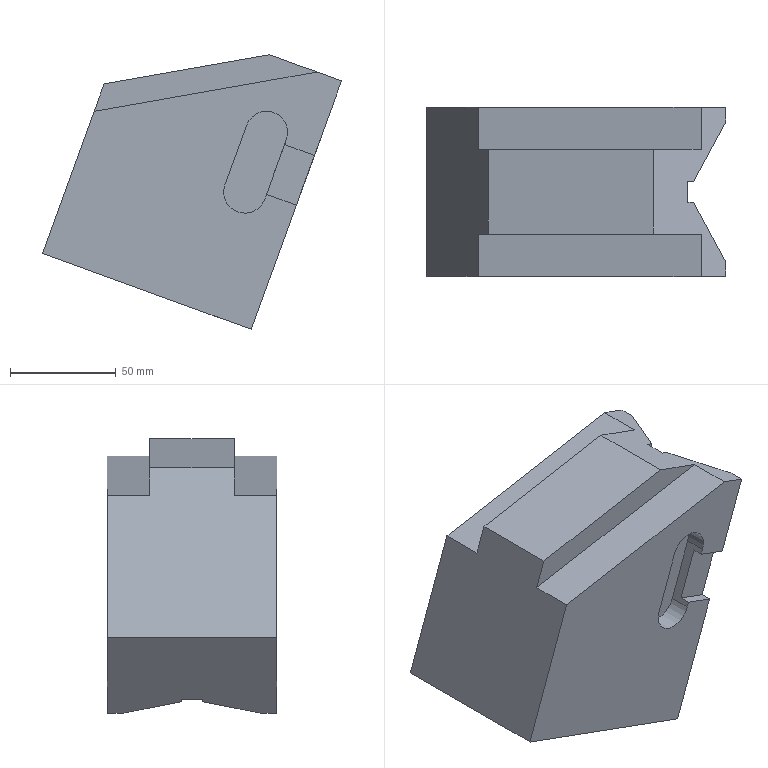Part | NX | features solid 2 | 1 solid | 33 faces | box 141.42 x 80 x 129.874 mm | volume 794242 mm3 | plane 29 | cylinder 4 | commonest cylinder face diameters 20 x4
STEP:
#1=CARTESIAN_POINT('',(813.449,-220.,121.531));
#2=VERTEX_POINT('',#1);
#3=CARTESIAN_POINT('',(828.59,-247.909,116.019));
#4=VERTEX_POINT('',#3);
#5=CARTESIAN_POINT('',(816.161,-225.,120.543));
#6=DIRECTION('',(0.4698,-0.866,-0.171));
#7=VECTOR('',#6,1000.);
#8=LINE('',#5,#7);
#9=EDGE_CURVE('',#2,#4,#8,.T.);
#10=ORIENTED_EDGE('',*,*,#9,.T.);
#11=CARTESIAN_POINT('',(785.838,-247.909,-1.442));
#12=VERTEX_POINT('',#11);
#13=CARTESIAN_POINT('',(837.141,-247.909,139.512));
#14=DIRECTION('',(-0.342,0.,-0.9397));
#15=VECTOR('',#14,1000.);
#16=LINE('',#13,#15);
#17=EDGE_CURVE('',#4,#12,#16,.T.);
#18=ORIENTED_EDGE('',*,*,#17,.T.);
#19=CARTESIAN_POINT('',(770.696,-220.,4.069));
#20=VERTEX_POINT('',#19);
#21=CARTESIAN_POINT('',(773.409,-225.,3.082));
#22=DIRECTION('',(0.4698,-0.866,-0.171));
#23=VECTOR('',#22,1000.);
#24=LINE('',#21,#23);
#25=EDGE_CURVE('',#20,#12,#24,.T.);
#26=ORIENTED_EDGE('',*,*,#25,.F.);
#27=CARTESIAN_POINT('',(821.999,-220.,145.023));
#28=DIRECTION('',(0.342,0.,0.9397));
#29=VECTOR('',#28,1000.);
#30=LINE('',#27,#29);
#31=EDGE_CURVE('',#20,#2,#30,.T.);
#32=ORIENTED_EDGE('',*,*,#31,.T.);
#33=EDGE_LOOP('',(#10,#18,#26,#32));
#34=FACE_BOUND('',#33,.T.);
#35=CARTESIAN_POINT('',(824.712,-225.,144.036));
#36=DIRECTION('',(0.8138,0.5,-0.2962));
#37=DIRECTION('',(0.342,0.,0.9397));
#38=AXIS2_PLACEMENT_3D('',#35,#36,#37);
#39=PLANE('',#38);
#40=ADVANCED_FACE('',(#34),#39,.T.);
#41=CARTESIAN_POINT('',(817.041,-175.,120.223));
#42=VERTEX_POINT('',#41);
#43=CARTESIAN_POINT('',(711.616,-175.,101.634));
#44=VERTEX_POINT('',#43);
#45=CARTESIAN_POINT('',(764.544,-175.,110.966));
#46=DIRECTION('',(-0.9848,0.,-0.1736));
#47=VECTOR('',#46,1000.);
#48=LINE('',#45,#47);
#49=EDGE_CURVE('',#42,#44,#48,.T.);
#50=ORIENTED_EDGE('',*,*,#49,.T.);
#51=CARTESIAN_POINT('',(711.616,-195.,101.634));
#52=VERTEX_POINT('',#51);
#53=CARTESIAN_POINT('',(711.616,-235.,101.634));
#54=DIRECTION('',(0.,1.,0.));
#55=VECTOR('',#54,1000.);
#56=LINE('',#53,#55);
#57=EDGE_CURVE('',#52,#44,#56,.T.);
#58=ORIENTED_EDGE('',*,*,#57,.F.);
#59=CARTESIAN_POINT('',(817.041,-195.,120.223));
#60=VERTEX_POINT('',#59);
#61=CARTESIAN_POINT('',(873.255,-195.,130.135));
#62=DIRECTION('',(0.9848,0.,0.1736));
#63=VECTOR('',#62,1000.);
#64=LINE('',#61,#63);
#65=EDGE_CURVE('',#60,#52,#64,.F.);
#66=ORIENTED_EDGE('',*,*,#65,.F.);
#67=CARTESIAN_POINT('',(817.041,-235.,120.223));
#68=DIRECTION('',(0.,-1.,0.));
#69=VECTOR('',#68,1000.);
#70=LINE('',#67,#69);
#71=EDGE_CURVE('',#42,#60,#70,.T.);
#72=ORIENTED_EDGE('',*,*,#71,.F.);
#73=EDGE_LOOP('',(#50,#58,#66,#72));
#74=FACE_BOUND('',#73,.T.);
#75=CARTESIAN_POINT('',(873.255,-235.,130.135));
#76=DIRECTION('',(0.1736,0.,-0.9848));
#77=DIRECTION('',(0.9848,0.,0.1736));
#78=AXIS2_PLACEMENT_3D('',#75,#76,#77);
#79=PLANE('',#78);
#80=ADVANCED_FACE('',(#74),#79,.F.);
#81=CARTESIAN_POINT('',(785.838,-175.,-1.442));
#82=VERTEX_POINT('',#81);
#83=CARTESIAN_POINT('',(687.17,-175.,34.47));
#84=VERTEX_POINT('',#83);
#85=CARTESIAN_POINT('',(781.139,-175.,0.268));
#86=DIRECTION('',(-0.9397,0.,0.342));
#87=VECTOR('',#86,1000.);
#88=LINE('',#85,#87);
#89=EDGE_CURVE('',#82,#84,#88,.T.);
#90=ORIENTED_EDGE('',*,*,#89,.F.);
#91=CARTESIAN_POINT('',(785.838,-182.091,-1.442));
#92=VERTEX_POINT('',#91);
#93=CARTESIAN_POINT('',(785.838,-175.,-1.442));
#94=DIRECTION('',(0.,1.,0.));
#95=VECTOR('',#94,1000.);
#96=LINE('',#93,#95);
#97=EDGE_CURVE('',#92,#82,#96,.T.);
#98=ORIENTED_EDGE('',*,*,#97,.F.);
#99=CARTESIAN_POINT('',(770.696,-210.,4.069));
#100=VERTEX_POINT('',#99);
#101=CARTESIAN_POINT('',(773.409,-205.,3.082));
#102=DIRECTION('',(0.4698,0.866,-0.171));
#103=VECTOR('',#102,1000.);
#104=LINE('',#101,#103);
#105=EDGE_CURVE('',#100,#92,#104,.T.);
#106=ORIENTED_EDGE('',*,*,#105,.F.);
#107=CARTESIAN_POINT('',(767.984,-210.,5.056));
#108=VERTEX_POINT('',#107);
#109=CARTESIAN_POINT('',(781.139,-210.,0.268));
#110=DIRECTION('',(0.9397,0.,-0.342));
#111=VECTOR('',#110,1000.);
#112=LINE('',#109,#111);
#113=EDGE_CURVE('',#108,#100,#112,.T.);
#114=ORIENTED_EDGE('',*,*,#113,.F.);
#115=CARTESIAN_POINT('',(767.984,-220.,5.056));
#116=VERTEX_POINT('',#115);
#117=CARTESIAN_POINT('',(767.984,-215.,5.056));
#118=DIRECTION('',(0.,1.,0.));
#119=VECTOR('',#118,1000.);
#120=LINE('',#117,#119);
#121=EDGE_CURVE('',#116,#108,#120,.T.);
#122=ORIENTED_EDGE('',*,*,#121,.F.);
#123=CARTESIAN_POINT('',(781.139,-220.,0.268));
#124=DIRECTION('',(0.9397,0.,-0.342));
#125=VECTOR('',#124,1000.);
#126=LINE('',#123,#125);
#127=EDGE_CURVE('',#116,#20,#126,.T.);
#128=ORIENTED_EDGE('',*,*,#127,.T.);
#129=ORIENTED_EDGE('',*,*,#25,.T.);
#130=CARTESIAN_POINT('',(785.838,-255.,-1.442));
#131=VERTEX_POINT('',#130);
#132=CARTESIAN_POINT('',(785.838,-255.,-1.442));
#133=DIRECTION('',(0.,-1.,0.));
#134=VECTOR('',#133,1000.);
#135=LINE('',#132,#134);
#136=EDGE_CURVE('',#12,#131,#135,.T.);
#137=ORIENTED_EDGE('',*,*,#136,.T.);
#138=CARTESIAN_POINT('',(687.17,-255.,34.47));
#139=VERTEX_POINT('',#138);
#140=CARTESIAN_POINT('',(781.139,-255.,0.268));
#141=DIRECTION('',(-0.9397,0.,0.342));
#142=VECTOR('',#141,1000.);
#143=LINE('',#140,#142);
#144=EDGE_CURVE('',#131,#139,#143,.T.);
#145=ORIENTED_EDGE('',*,*,#144,.T.);
#146=CARTESIAN_POINT('',(687.17,-215.,34.47));
#147=DIRECTION('',(0.,-1.,0.));
#148=VECTOR('',#147,1000.);
#149=LINE('',#146,#148);
#150=EDGE_CURVE('',#84,#139,#149,.T.);
#151=ORIENTED_EDGE('',*,*,#150,.F.);
#152=EDGE_LOOP('',(#90,#98,#106,#114,#122,#128,#129,#137,#145,#151));
#153=FACE_BOUND('',#152,.T.);
#154=CARTESIAN_POINT('',(781.139,-215.,0.268));
#155=DIRECTION('',(-0.342,0.,-0.9397));
#156=DIRECTION('',(0.9397,0.,-0.342));
#157=AXIS2_PLACEMENT_3D('',#154,#155,#156);
#158=PLANE('',#157);
#159=ADVANCED_FACE('',(#153),#158,.T.);
#160=CARTESIAN_POINT('',(817.041,-255.,120.223));
#161=VERTEX_POINT('',#160);
#162=CARTESIAN_POINT('',(711.616,-255.,101.634));
#163=VERTEX_POINT('',#162);
#164=CARTESIAN_POINT('',(873.255,-255.,130.135));
#165=DIRECTION('',(-0.9848,0.,-0.1736));
#166=VECTOR('',#165,1000.);
#167=LINE('',#164,#166);
#168=EDGE_CURVE('',#161,#163,#167,.T.);
#169=ORIENTED_EDGE('',*,*,#168,.T.);
#170=CARTESIAN_POINT('',(713.455,-255.,106.689));
#171=DIRECTION('',(0.342,0.,0.9397));
#172=VECTOR('',#171,1000.);
#173=LINE('',#170,#172);
#174=EDGE_CURVE('',#139,#163,#173,.T.);
#175=ORIENTED_EDGE('',*,*,#174,.F.);
#176=ORIENTED_EDGE('',*,*,#144,.F.);
#177=CARTESIAN_POINT('',(807.214,-255.,57.289));
#178=VERTEX_POINT('',#177);
#179=CARTESIAN_POINT('',(812.123,-255.,70.777));
#180=DIRECTION('',(-0.342,0.,-0.9397));
#181=VECTOR('',#180,1000.);
#182=LINE('',#179,#181);
#183=EDGE_CURVE('',#178,#131,#182,.T.);
#184=ORIENTED_EDGE('',*,*,#183,.F.);
#185=CARTESIAN_POINT('',(793.119,-255.,62.419));
#186=VERTEX_POINT('',#185);
#187=CARTESIAN_POINT('',(810.033,-255.,56.263));
#188=DIRECTION('',(-0.9397,0.,0.342));
#189=VECTOR('',#188,1000.);
#190=LINE('',#187,#189);
#191=EDGE_CURVE('',#178,#186,#190,.T.);
#192=ORIENTED_EDGE('',*,*,#191,.T.);
#193=CARTESIAN_POINT('',(792.264,-255.,60.07));
#194=VERTEX_POINT('',#193);
#195=CARTESIAN_POINT('',(797.394,-255.,74.165));
#196=DIRECTION('',(-0.342,0.,-0.9397));
#197=VECTOR('',#196,1000.);
#198=LINE('',#195,#197);
#199=EDGE_CURVE('',#186,#194,#198,.T.);
#200=ORIENTED_EDGE('',*,*,#199,.T.);
#201=CARTESIAN_POINT('',(773.47,-255.,66.91));
#202=VERTEX_POINT('',#201);
#203=CARTESIAN_POINT('',(782.867,-255.,63.49));
#204=DIRECTION('',(0.,1.,0.));
#205=DIRECTION('',(0.8192,0.,-0.5736));
#206=AXIS2_PLACEMENT_3D('',#203,#204,#205);
#207=CIRCLE('',#206,10.);
#208=EDGE_CURVE('',#194,#202,#207,.T.);
#209=ORIENTED_EDGE('',*,*,#208,.T.);
#210=CARTESIAN_POINT('',(783.73,-255.,95.101));
#211=VERTEX_POINT('',#210);
#212=CARTESIAN_POINT('',(778.6,-255.,81.006));
#213=DIRECTION('',(-0.342,0.,-0.9397));
#214=VECTOR('',#213,1000.);
#215=LINE('',#212,#214);
#216=EDGE_CURVE('',#211,#202,#215,.T.);
#217=ORIENTED_EDGE('',*,*,#216,.F.);
#218=CARTESIAN_POINT('',(802.524,-255.,88.261));
#219=VERTEX_POINT('',#218);
#220=CARTESIAN_POINT('',(793.127,-255.,91.681));
#221=DIRECTION('',(0.,1.,0.));
#222=DIRECTION('',(0.8192,0.,-0.5736));
#223=AXIS2_PLACEMENT_3D('',#220,#221,#222);
#224=CIRCLE('',#223,10.);
#225=EDGE_CURVE('',#211,#219,#224,.T.);
#226=ORIENTED_EDGE('',*,*,#225,.T.);
#227=CARTESIAN_POINT('',(801.669,-255.,85.911));
#228=VERTEX_POINT('',#227);
#229=CARTESIAN_POINT('',(797.394,-255.,74.165));
#230=DIRECTION('',(-0.342,0.,-0.9397));
#231=VECTOR('',#230,1000.);
#232=LINE('',#229,#231);
#233=EDGE_CURVE('',#219,#228,#232,.T.);
#234=ORIENTED_EDGE('',*,*,#233,.T.);
#235=CARTESIAN_POINT('',(815.764,-255.,80.781));
#236=VERTEX_POINT('',#235);
#237=CARTESIAN_POINT('',(818.584,-255.,79.755));
#238=DIRECTION('',(-0.9397,0.,0.342));
#239=VECTOR('',#238,1000.);
#240=LINE('',#237,#239);
#241=EDGE_CURVE('',#236,#228,#240,.T.);
#242=ORIENTED_EDGE('',*,*,#241,.F.);
#243=CARTESIAN_POINT('',(828.59,-255.,116.019));
#244=VERTEX_POINT('',#243);
#245=CARTESIAN_POINT('',(812.123,-255.,70.777));
#246=DIRECTION('',(-0.342,0.,-0.9397));
#247=VECTOR('',#246,1000.);
#248=LINE('',#245,#247);
#249=EDGE_CURVE('',#244,#236,#248,.T.);
#250=ORIENTED_EDGE('',*,*,#249,.F.);
#251=CARTESIAN_POINT('',(823.892,-255.,117.73));
#252=DIRECTION('',(-0.9397,0.,0.342));
#253=VECTOR('',#252,1000.);
#254=LINE('',#251,#253);
#255=EDGE_CURVE('',#244,#161,#254,.T.);
#256=ORIENTED_EDGE('',*,*,#255,.T.);
#257=EDGE_LOOP('',(#169,#175,#176,#184,#192,#200,#209,#217,#226,#234,#242,#250,#256));
#258=FACE_BOUND('',#257,.T.);
#259=CARTESIAN_POINT('',(768.854,-255.,86.525));
#260=DIRECTION('',(0.,1.,0.));
#261=DIRECTION('',(-0.8192,0.,0.5736));
#262=AXIS2_PLACEMENT_3D('',#259,#260,#261);
#263=PLANE('',#262);
#264=ADVANCED_FACE('',(#258),#263,.F.);
#265=CARTESIAN_POINT('',(828.59,-175.,116.019));
#266=VERTEX_POINT('',#265);
#267=CARTESIAN_POINT('',(815.764,-175.,80.781));
#268=VERTEX_POINT('',#267);
#269=CARTESIAN_POINT('',(812.123,-175.,70.777));
#270=DIRECTION('',(-0.342,0.,-0.9397));
#271=VECTOR('',#270,1000.);
#272=LINE('',#269,#271);
#273=EDGE_CURVE('',#266,#268,#272,.T.);
#274=ORIENTED_EDGE('',*,*,#273,.T.);
#275=CARTESIAN_POINT('',(801.669,-175.,85.911));
#276=VERTEX_POINT('',#275);
#277=CARTESIAN_POINT('',(818.584,-175.,79.755));
#278=DIRECTION('',(-0.9397,0.,0.342));
#279=VECTOR('',#278,1000.);
#280=LINE('',#277,#279);
#281=EDGE_CURVE('',#268,#276,#280,.T.);
#282=ORIENTED_EDGE('',*,*,#281,.T.);
#283=CARTESIAN_POINT('',(802.524,-175.,88.261));
#284=VERTEX_POINT('',#283);
#285=CARTESIAN_POINT('',(797.394,-175.,74.165));
#286=DIRECTION('',(-0.342,0.,-0.9397));
#287=VECTOR('',#286,1000.);
#288=LINE('',#285,#287);
#289=EDGE_CURVE('',#284,#276,#288,.T.);
#290=ORIENTED_EDGE('',*,*,#289,.F.);
#291=CARTESIAN_POINT('',(783.73,-175.,95.101));
#292=VERTEX_POINT('',#291);
#293=CARTESIAN_POINT('',(793.127,-175.,91.681));
#294=DIRECTION('',(0.,1.,0.));
#295=DIRECTION('',(0.8192,0.,-0.5736));
#296=AXIS2_PLACEMENT_3D('',#293,#294,#295);
#297=CIRCLE('',#296,10.);
#298=EDGE_CURVE('',#292,#284,#297,.T.);
#299=ORIENTED_EDGE('',*,*,#298,.F.);
#300=CARTESIAN_POINT('',(773.47,-175.,66.91));
#301=VERTEX_POINT('',#300);
#302=CARTESIAN_POINT('',(778.6,-175.,81.006));
#303=DIRECTION('',(-0.342,0.,-0.9397));
#304=VECTOR('',#303,1000.);
#305=LINE('',#302,#304);
#306=EDGE_CURVE('',#292,#301,#305,.T.);
#307=ORIENTED_EDGE('',*,*,#306,.T.);
#308=CARTESIAN_POINT('',(792.264,-175.,60.07));
#309=VERTEX_POINT('',#308);
#310=CARTESIAN_POINT('',(782.867,-175.,63.49));
#311=DIRECTION('',(0.,1.,0.));
#312=DIRECTION('',(0.8192,0.,-0.5736));
#313=AXIS2_PLACEMENT_3D('',#310,#311,#312);
#314=CIRCLE('',#313,10.);
#315=EDGE_CURVE('',#309,#301,#314,.T.);
#316=ORIENTED_EDGE('',*,*,#315,.F.);
#317=CARTESIAN_POINT('',(793.119,-175.,62.419));
#318=VERTEX_POINT('',#317);
#319=CARTESIAN_POINT('',(797.394,-175.,74.165));
#320=DIRECTION('',(-0.342,0.,-0.9397));
#321=VECTOR('',#320,1000.);
#322=LINE('',#319,#321);
#323=EDGE_CURVE('',#318,#309,#322,.T.);
#324=ORIENTED_EDGE('',*,*,#323,.F.);
#325=CARTESIAN_POINT('',(807.214,-175.,57.289));
#326=VERTEX_POINT('',#325);
#327=CARTESIAN_POINT('',(810.033,-175.,56.263));
#328=DIRECTION('',(-0.9397,0.,0.342));
#329=VECTOR('',#328,1000.);
#330=LINE('',#327,#329);
#331=EDGE_CURVE('',#326,#318,#330,.T.);
#332=ORIENTED_EDGE('',*,*,#331,.F.);
#333=CARTESIAN_POINT('',(812.123,-175.,70.777));
#334=DIRECTION('',(-0.342,0.,-0.9397));
#335=VECTOR('',#334,1000.);
#336=LINE('',#333,#335);
#337=EDGE_CURVE('',#326,#82,#336,.T.);
#338=ORIENTED_EDGE('',*,*,#337,.T.);
#339=ORIENTED_EDGE('',*,*,#89,.T.);
#340=CARTESIAN_POINT('',(713.455,-175.,106.689));
#341=DIRECTION('',(-0.342,0.,-0.9397));
#342=VECTOR('',#341,1000.);
#343=LINE('',#340,#342);
#344=EDGE_CURVE('',#44,#84,#343,.T.);
#345=ORIENTED_EDGE('',*,*,#344,.F.);
#346=ORIENTED_EDGE('',*,*,#49,.F.);
#347=CARTESIAN_POINT('',(823.892,-175.,117.73));
#348=DIRECTION('',(-0.9397,0.,0.342));
#349=VECTOR('',#348,1000.);
#350=LINE('',#347,#349);
#351=EDGE_CURVE('',#266,#42,#350,.T.);
#352=ORIENTED_EDGE('',*,*,#351,.F.);
#353=EDGE_LOOP('',(#274,#282,#290,#299,#307,#316,#324,#332,#338,#339,#345,#346,#352));
#354=FACE_BOUND('',#353,.T.);
#355=CARTESIAN_POINT('',(768.854,-175.,86.525));
#356=DIRECTION('',(0.,-1.,0.));
#357=DIRECTION('',(-0.8192,0.,0.5736));
#358=AXIS2_PLACEMENT_3D('',#355,#356,#357);
#359=PLANE('',#358);
#360=ADVANCED_FACE('',(#354),#359,.F.);
#361=ORIENTED_EDGE('',*,*,#249,.T.);
#362=CARTESIAN_POINT('',(815.764,-250.,80.781));
#363=VERTEX_POINT('',#362);
#364=CARTESIAN_POINT('',(815.764,-255.,80.781));
#365=DIRECTION('',(0.,-1.,0.));
#366=VECTOR('',#365,1000.);
#367=LINE('',#364,#366);
#368=EDGE_CURVE('',#363,#236,#367,.T.);
#369=ORIENTED_EDGE('',*,*,#368,.F.);
#370=CARTESIAN_POINT('',(807.214,-250.,57.289));
#371=VERTEX_POINT('',#370);
#372=CARTESIAN_POINT('',(835.431,-250.,134.813));
#373=DIRECTION('',(0.342,0.,0.9397));
#374=VECTOR('',#373,1000.);
#375=LINE('',#372,#374);
#376=EDGE_CURVE('',#371,#363,#375,.T.);
#377=ORIENTED_EDGE('',*,*,#376,.F.);
#378=CARTESIAN_POINT('',(807.214,-255.,57.289));
#379=DIRECTION('',(0.,1.,0.));
#380=VECTOR('',#379,1000.);
#381=LINE('',#378,#380);
#382=EDGE_CURVE('',#178,#371,#381,.T.);
#383=ORIENTED_EDGE('',*,*,#382,.F.);
#384=ORIENTED_EDGE('',*,*,#183,.T.);
#385=ORIENTED_EDGE('',*,*,#136,.F.);
#386=ORIENTED_EDGE('',*,*,#17,.F.);
#387=CARTESIAN_POINT('',(828.59,-255.,116.019));
#388=DIRECTION('',(0.,-1.,0.));
#389=VECTOR('',#388,1000.);
#390=LINE('',#387,#389);
#391=EDGE_CURVE('',#4,#244,#390,.T.);
#392=ORIENTED_EDGE('',*,*,#391,.T.);
#393=EDGE_LOOP('',(#361,#369,#377,#383,#384,#385,#386,#392));
#394=FACE_BOUND('',#393,.T.);
#395=CARTESIAN_POINT('',(837.141,-255.,139.512));
#396=DIRECTION('',(-0.9397,0.,0.342));
#397=DIRECTION('',(-0.342,0.,-0.9397));
#398=AXIS2_PLACEMENT_3D('',#395,#396,#397);
#399=PLANE('',#398);
#400=ADVANCED_FACE('',(#394),#399,.F.);
#401=ORIENTED_EDGE('',*,*,#216,.T.);
#402=CARTESIAN_POINT('',(773.47,-245.,66.91));
#403=VERTEX_POINT('',#402);
#404=CARTESIAN_POINT('',(773.47,-255.,66.91));
#405=DIRECTION('',(0.,-1.,0.));
#406=VECTOR('',#405,1000.);
#407=LINE('',#404,#406);
#408=EDGE_CURVE('',#403,#202,#407,.T.);
#409=ORIENTED_EDGE('',*,*,#408,.F.);
#410=CARTESIAN_POINT('',(783.73,-245.,95.101));
#411=VERTEX_POINT('',#410);
#412=CARTESIAN_POINT('',(783.73,-245.,95.101));
#413=DIRECTION('',(-0.342,0.,-0.9397));
#414=VECTOR('',#413,1000.);
#415=LINE('',#412,#414);
#416=EDGE_CURVE('',#411,#403,#415,.T.);
#417=ORIENTED_EDGE('',*,*,#416,.F.);
#418=CARTESIAN_POINT('',(783.73,-255.,95.101));
#419=DIRECTION('',(0.,-1.,0.));
#420=VECTOR('',#419,1000.);
#421=LINE('',#418,#420);
#422=EDGE_CURVE('',#411,#211,#421,.T.);
#423=ORIENTED_EDGE('',*,*,#422,.T.);
#424=EDGE_LOOP('',(#401,#409,#417,#423));
#425=FACE_BOUND('',#424,.T.);
#426=CARTESIAN_POINT('',(778.6,-255.,81.006));
#427=DIRECTION('',(-0.9397,0.,0.342));
#428=DIRECTION('',(-0.342,0.,-0.9397));
#429=AXIS2_PLACEMENT_3D('',#426,#427,#428);
#430=PLANE('',#429);
#431=ADVANCED_FACE('',(#425),#430,.F.);
#432=ORIENTED_EDGE('',*,*,#416,.T.);
#433=CARTESIAN_POINT('',(792.264,-245.,60.07));
#434=VERTEX_POINT('',#433);
#435=CARTESIAN_POINT('',(782.867,-245.,63.49));
#436=DIRECTION('',(0.,1.,0.));
#437=DIRECTION('',(0.8192,0.,-0.5736));
#438=AXIS2_PLACEMENT_3D('',#435,#436,#437);
#439=CIRCLE('',#438,10.);
#440=EDGE_CURVE('',#434,#403,#439,.T.);
#441=ORIENTED_EDGE('',*,*,#440,.F.);
#442=CARTESIAN_POINT('',(802.524,-245.,88.261));
#443=VERTEX_POINT('',#442);
#444=CARTESIAN_POINT('',(802.524,-245.,88.261));
#445=DIRECTION('',(-0.342,0.,-0.9397));
#446=VECTOR('',#445,1000.);
#447=LINE('',#444,#446);
#448=EDGE_CURVE('',#443,#434,#447,.T.);
#449=ORIENTED_EDGE('',*,*,#448,.F.);
#450=CARTESIAN_POINT('',(793.127,-245.,91.681));
#451=DIRECTION('',(0.,1.,0.));
#452=DIRECTION('',(0.8192,0.,-0.5736));
#453=AXIS2_PLACEMENT_3D('',#450,#451,#452);
#454=CIRCLE('',#453,10.);
#455=EDGE_CURVE('',#411,#443,#454,.T.);
#456=ORIENTED_EDGE('',*,*,#455,.F.);
#457=EDGE_LOOP('',(#432,#441,#449,#456));
#458=FACE_BOUND('',#457,.T.);
#459=CARTESIAN_POINT('',(787.997,-245.,77.585));
#460=DIRECTION('',(0.,1.,0.));
#461=DIRECTION('',(-0.8192,0.,0.5736));
#462=AXIS2_PLACEMENT_3D('',#459,#460,#461);
#463=PLANE('',#462);
#464=ADVANCED_FACE('',(#458),#463,.F.);
#465=ORIENTED_EDGE('',*,*,#225,.F.);
#466=ORIENTED_EDGE('',*,*,#422,.F.);
#467=ORIENTED_EDGE('',*,*,#455,.T.);
#468=CARTESIAN_POINT('',(802.524,-255.,88.261));
#469=DIRECTION('',(0.,-1.,0.));
#470=VECTOR('',#469,1000.);
#471=LINE('',#468,#470);
#472=EDGE_CURVE('',#443,#219,#471,.T.);
#473=ORIENTED_EDGE('',*,*,#472,.T.);
#474=EDGE_LOOP('',(#465,#466,#467,#473));
#475=FACE_BOUND('',#474,.T.);
#476=CARTESIAN_POINT('',(793.127,-255.,91.681));
#477=DIRECTION('',(0.,-1.,0.));
#478=DIRECTION('',(0.8192,0.,-0.5736));
#479=AXIS2_PLACEMENT_3D('',#476,#477,#478);
#480=CYLINDRICAL_SURFACE('',#479,10.);
#481=ADVANCED_FACE('',(#475),#480,.F.);
#482=CARTESIAN_POINT('',(801.669,-250.,85.911));
#483=VERTEX_POINT('',#482);
#484=CARTESIAN_POINT('',(793.119,-250.,62.419));
#485=VERTEX_POINT('',#484);
#486=CARTESIAN_POINT('',(795.684,-250.,69.467));
#487=DIRECTION('',(-0.342,0.,-0.9397));
#488=VECTOR('',#487,1000.);
#489=LINE('',#486,#488);
#490=EDGE_CURVE('',#483,#485,#489,.T.);
#491=ORIENTED_EDGE('',*,*,#490,.F.);
#492=CARTESIAN_POINT('',(801.669,-255.,85.911));
#493=DIRECTION('',(0.,1.,0.));
#494=VECTOR('',#493,1000.);
#495=LINE('',#492,#494);
#496=EDGE_CURVE('',#228,#483,#495,.T.);
#497=ORIENTED_EDGE('',*,*,#496,.F.);
#498=ORIENTED_EDGE('',*,*,#233,.F.);
#499=ORIENTED_EDGE('',*,*,#472,.F.);
#500=ORIENTED_EDGE('',*,*,#448,.T.);
#501=CARTESIAN_POINT('',(792.264,-255.,60.07));
#502=DIRECTION('',(0.,-1.,0.));
#503=VECTOR('',#502,1000.);
#504=LINE('',#501,#503);
#505=EDGE_CURVE('',#434,#194,#504,.T.);
#506=ORIENTED_EDGE('',*,*,#505,.T.);
#507=ORIENTED_EDGE('',*,*,#199,.F.);
#508=CARTESIAN_POINT('',(793.119,-255.,62.419));
#509=DIRECTION('',(0.,-1.,0.));
#510=VECTOR('',#509,1000.);
#511=LINE('',#508,#510);
#512=EDGE_CURVE('',#485,#186,#511,.T.);
#513=ORIENTED_EDGE('',*,*,#512,.F.);
#514=EDGE_LOOP('',(#491,#497,#498,#499,#500,#506,#507,#513));
#515=FACE_BOUND('',#514,.T.);
#516=CARTESIAN_POINT('',(797.394,-255.,74.165));
#517=DIRECTION('',(0.9397,0.,-0.342));
#518=DIRECTION('',(0.342,0.,0.9397));
#519=AXIS2_PLACEMENT_3D('',#516,#517,#518);
#520=PLANE('',#519);
#521=ADVANCED_FACE('',(#515),#520,.F.);
#522=ORIENTED_EDGE('',*,*,#208,.F.);
#523=ORIENTED_EDGE('',*,*,#505,.F.);
#524=ORIENTED_EDGE('',*,*,#440,.T.);
#525=ORIENTED_EDGE('',*,*,#408,.T.);
#526=EDGE_LOOP('',(#522,#523,#524,#525));
#527=FACE_BOUND('',#526,.T.);
#528=CARTESIAN_POINT('',(782.867,-255.,63.49));
#529=DIRECTION('',(0.,-1.,0.));
#530=DIRECTION('',(0.8192,0.,-0.5736));
#531=AXIS2_PLACEMENT_3D('',#528,#529,#530);
#532=CYLINDRICAL_SURFACE('',#531,10.);
#533=ADVANCED_FACE('',(#527),#532,.F.);
#534=ORIENTED_EDGE('',*,*,#191,.F.);
#535=ORIENTED_EDGE('',*,*,#382,.T.);
#536=CARTESIAN_POINT('',(810.033,-250.,56.263));
#537=DIRECTION('',(-0.9397,0.,0.342));
#538=VECTOR('',#537,1000.);
#539=LINE('',#536,#538);
#540=EDGE_CURVE('',#371,#485,#539,.T.);
#541=ORIENTED_EDGE('',*,*,#540,.T.);
#542=ORIENTED_EDGE('',*,*,#512,.T.);
#543=EDGE_LOOP('',(#534,#535,#541,#542));
#544=FACE_BOUND('',#543,.T.);
#545=CARTESIAN_POINT('',(810.033,-255.,56.263));
#546=DIRECTION('',(-0.342,0.,-0.9397));
#547=DIRECTION('',(0.9397,0.,-0.342));
#548=AXIS2_PLACEMENT_3D('',#545,#546,#547);
#549=PLANE('',#548);
#550=ADVANCED_FACE('',(#544),#549,.F.);
#551=ORIENTED_EDGE('',*,*,#540,.F.);
#552=ORIENTED_EDGE('',*,*,#376,.T.);
#553=CARTESIAN_POINT('',(818.584,-250.,79.755));
#554=DIRECTION('',(-0.9397,0.,0.342));
#555=VECTOR('',#554,1000.);
#556=LINE('',#553,#555);
#557=EDGE_CURVE('',#363,#483,#556,.T.);
#558=ORIENTED_EDGE('',*,*,#557,.T.);
#559=ORIENTED_EDGE('',*,*,#490,.T.);
#560=EDGE_LOOP('',(#551,#552,#558,#559));
#561=FACE_BOUND('',#560,.T.);
#562=CARTESIAN_POINT('',(816.873,-250.,75.056));
#563=DIRECTION('',(0.,1.,0.));
#564=DIRECTION('',(-0.8192,0.,0.5736));
#565=AXIS2_PLACEMENT_3D('',#562,#563,#564);
#566=PLANE('',#565);
#567=ADVANCED_FACE('',(#561),#566,.F.);
#568=ORIENTED_EDGE('',*,*,#557,.F.);
#569=ORIENTED_EDGE('',*,*,#368,.T.);
#570=ORIENTED_EDGE('',*,*,#241,.T.);
#571=ORIENTED_EDGE('',*,*,#496,.T.);
#572=EDGE_LOOP('',(#568,#569,#570,#571));
#573=FACE_BOUND('',#572,.T.);
#574=CARTESIAN_POINT('',(799.79,-255.,86.595));
#575=DIRECTION('',(0.342,0.,0.9397));
#576=DIRECTION('',(-0.9397,0.,0.342));
#577=AXIS2_PLACEMENT_3D('',#574,#575,#576);
#578=PLANE('',#577);
#579=ADVANCED_FACE('',(#573),#578,.F.);
#580=CARTESIAN_POINT('',(817.041,-235.,120.223));
#581=VERTEX_POINT('',#580);
#582=CARTESIAN_POINT('',(794.489,-235.,128.431));
#583=VERTEX_POINT('',#582);
#584=CARTESIAN_POINT('',(849.706,-235.,108.334));
#585=DIRECTION('',(0.9397,0.,-0.342));
#586=VECTOR('',#585,1000.);
#587=LINE('',#584,#586);
#588=EDGE_CURVE('',#581,#583,#587,.F.);
#589=ORIENTED_EDGE('',*,*,#588,.T.);
#590=CARTESIAN_POINT('',(716.355,-235.,114.654));
#591=VERTEX_POINT('',#590);
#592=CARTESIAN_POINT('',(868.344,-235.,141.454));
#593=DIRECTION('',(0.9848,0.,0.1736));
#594=VECTOR('',#593,1000.);
#595=LINE('',#592,#594);
#596=EDGE_CURVE('',#583,#591,#595,.F.);
#597=ORIENTED_EDGE('',*,*,#596,.T.);
#598=CARTESIAN_POINT('',(711.616,-235.,101.634));
#599=VERTEX_POINT('',#598);
#600=CARTESIAN_POINT('',(746.412,-235.,197.235));
#601=DIRECTION('',(0.342,0.,0.9397));
#602=VECTOR('',#601,1000.);
#603=LINE('',#600,#602);
#604=EDGE_CURVE('',#591,#599,#603,.F.);
#605=ORIENTED_EDGE('',*,*,#604,.T.);
#606=CARTESIAN_POINT('',(870.427,-235.,129.636));
#607=DIRECTION('',(0.9848,0.,0.1736));
#608=VECTOR('',#607,1000.);
#609=LINE('',#606,#608);
#610=EDGE_CURVE('',#581,#599,#609,.F.);
#611=ORIENTED_EDGE('',*,*,#610,.F.);
#612=EDGE_LOOP('',(#589,#597,#605,#611));
#613=FACE_BOUND('',#612,.T.);
#614=CARTESIAN_POINT('',(866.195,-235.,153.638));
#615=DIRECTION('',(0.,1.,0.));
#616=DIRECTION('',(-0.9659,0.,-0.2588));
#617=AXIS2_PLACEMENT_3D('',#614,#615,#616);
#618=PLANE('',#617);
#619=ADVANCED_FACE('',(#613),#618,.F.);
#620=ORIENTED_EDGE('',*,*,#610,.T.);
#621=CARTESIAN_POINT('',(711.616,-235.,101.634));
#622=DIRECTION('',(0.,1.,0.));
#623=VECTOR('',#622,1000.);
#624=LINE('',#621,#623);
#625=EDGE_CURVE('',#163,#599,#624,.T.);
#626=ORIENTED_EDGE('',*,*,#625,.F.);
#627=ORIENTED_EDGE('',*,*,#168,.F.);
#628=CARTESIAN_POINT('',(817.041,-235.,120.223));
#629=DIRECTION('',(0.,-1.,0.));
#630=VECTOR('',#629,1000.);
#631=LINE('',#628,#630);
#632=EDGE_CURVE('',#581,#161,#631,.T.);
#633=ORIENTED_EDGE('',*,*,#632,.F.);
#634=EDGE_LOOP('',(#620,#626,#627,#633));
#635=FACE_BOUND('',#634,.T.);
#636=CARTESIAN_POINT('',(873.255,-235.,130.135));
#637=DIRECTION('',(0.1736,0.,-0.9848));
#638=DIRECTION('',(0.9848,0.,0.1736));
#639=AXIS2_PLACEMENT_3D('',#636,#637,#638);
#640=PLANE('',#639);
#641=ADVANCED_FACE('',(#635),#640,.F.);
#642=ORIENTED_EDGE('',*,*,#31,.F.);
#643=ORIENTED_EDGE('',*,*,#127,.F.);
#644=CARTESIAN_POINT('',(810.736,-220.,122.518));
#645=VERTEX_POINT('',#644);
#646=CARTESIAN_POINT('',(817.294,-220.,140.534));
#647=DIRECTION('',(-0.342,0.,-0.9397));
#648=VECTOR('',#647,1000.);
#649=LINE('',#646,#648);
#650=EDGE_CURVE('',#645,#116,#649,.T.);
#651=ORIENTED_EDGE('',*,*,#650,.F.);
#652=CARTESIAN_POINT('',(823.892,-220.,117.73));
#653=DIRECTION('',(0.9397,0.,-0.342));
#654=VECTOR('',#653,1000.);
#655=LINE('',#652,#654);
#656=EDGE_CURVE('',#645,#2,#655,.T.);
#657=ORIENTED_EDGE('',*,*,#656,.T.);
#658=EDGE_LOOP('',(#642,#643,#651,#657));
#659=FACE_BOUND('',#658,.T.);
#660=CARTESIAN_POINT('',(826.691,-220.,137.114));
#661=DIRECTION('',(0.,-1.,0.));
#662=DIRECTION('',(0.8192,0.,-0.5736));
#663=AXIS2_PLACEMENT_3D('',#660,#661,#662);
#664=PLANE('',#663);
#665=ADVANCED_FACE('',(#659),#664,.F.);
#666=CARTESIAN_POINT('',(810.736,-210.,122.518));
#667=VERTEX_POINT('',#666);
#668=CARTESIAN_POINT('',(810.736,-215.,122.518));
#669=DIRECTION('',(0.,1.,0.));
#670=VECTOR('',#669,1000.);
#671=LINE('',#668,#670);
#672=EDGE_CURVE('',#645,#667,#671,.T.);
#673=ORIENTED_EDGE('',*,*,#672,.F.);
#674=ORIENTED_EDGE('',*,*,#650,.T.);
#675=ORIENTED_EDGE('',*,*,#121,.T.);
#676=CARTESIAN_POINT('',(817.294,-210.,140.534));
#677=DIRECTION('',(-0.342,0.,-0.9397));
#678=VECTOR('',#677,1000.);
#679=LINE('',#676,#678);
#680=EDGE_CURVE('',#667,#108,#679,.T.);
#681=ORIENTED_EDGE('',*,*,#680,.F.);
#682=EDGE_LOOP('',(#673,#674,#675,#681));
#683=FACE_BOUND('',#682,.T.);
#684=CARTESIAN_POINT('',(817.294,-215.,140.534));
#685=DIRECTION('',(0.9397,0.,-0.342));
#686=DIRECTION('',(-0.342,0.,-0.9397));
#687=AXIS2_PLACEMENT_3D('',#684,#685,#686);
#688=PLANE('',#687);
#689=ADVANCED_FACE('',(#683),#688,.T.);
#690=CARTESIAN_POINT('',(813.449,-210.,121.531));
#691=VERTEX_POINT('',#690);
#692=CARTESIAN_POINT('',(828.59,-182.091,116.019));
#693=VERTEX_POINT('',#692);
#694=CARTESIAN_POINT('',(816.161,-205.,120.543));
#695=DIRECTION('',(0.4698,0.866,-0.171));
#696=VECTOR('',#695,1000.);
#697=LINE('',#694,#696);
#698=EDGE_CURVE('',#691,#693,#697,.T.);
#699=ORIENTED_EDGE('',*,*,#698,.F.);
#700=CARTESIAN_POINT('',(821.999,-210.,145.023));
#701=DIRECTION('',(0.342,0.,0.9397));
#702=VECTOR('',#701,1000.);
#703=LINE('',#700,#702);
#704=EDGE_CURVE('',#100,#691,#703,.T.);
#705=ORIENTED_EDGE('',*,*,#704,.F.);
#706=ORIENTED_EDGE('',*,*,#105,.T.);
#707=CARTESIAN_POINT('',(837.141,-182.091,139.512));
#708=DIRECTION('',(-0.342,0.,-0.9397));
#709=VECTOR('',#708,1000.);
#710=LINE('',#707,#709);
#711=EDGE_CURVE('',#693,#92,#710,.T.);
#712=ORIENTED_EDGE('',*,*,#711,.F.);
#713=EDGE_LOOP('',(#699,#705,#706,#712));
#714=FACE_BOUND('',#713,.T.);
#715=CARTESIAN_POINT('',(824.712,-205.,144.036));
#716=DIRECTION('',(0.8138,-0.5,-0.2962));
#717=DIRECTION('',(0.342,0.,0.9397));
#718=AXIS2_PLACEMENT_3D('',#715,#716,#717);
#719=PLANE('',#718);
#720=ADVANCED_FACE('',(#714),#719,.T.);
#721=ORIENTED_EDGE('',*,*,#711,.T.);
#722=ORIENTED_EDGE('',*,*,#97,.T.);
#723=ORIENTED_EDGE('',*,*,#337,.F.);
#724=CARTESIAN_POINT('',(807.214,-180.,57.289));
#725=VERTEX_POINT('',#724);
#726=CARTESIAN_POINT('',(807.214,-175.,57.289));
#727=DIRECTION('',(0.,-1.,0.));
#728=VECTOR('',#727,1000.);
#729=LINE('',#726,#728);
#730=EDGE_CURVE('',#326,#725,#729,.T.);
#731=ORIENTED_EDGE('',*,*,#730,.T.);
#732=CARTESIAN_POINT('',(815.764,-180.,80.781));
#733=VERTEX_POINT('',#732);
#734=CARTESIAN_POINT('',(837.141,-180.,139.512));
#735=DIRECTION('',(0.342,0.,0.9397));
#736=VECTOR('',#735,1000.);
#737=LINE('',#734,#736);
#738=EDGE_CURVE('',#725,#733,#737,.T.);
#739=ORIENTED_EDGE('',*,*,#738,.T.);
#740=CARTESIAN_POINT('',(815.764,-175.,80.781));
#741=DIRECTION('',(0.,1.,0.));
#742=VECTOR('',#741,1000.);
#743=LINE('',#740,#742);
#744=EDGE_CURVE('',#733,#268,#743,.T.);
#745=ORIENTED_EDGE('',*,*,#744,.T.);
#746=ORIENTED_EDGE('',*,*,#273,.F.);
#747=CARTESIAN_POINT('',(828.59,-175.,116.019));
#748=DIRECTION('',(0.,1.,0.));
#749=VECTOR('',#748,1000.);
#750=LINE('',#747,#749);
#751=EDGE_CURVE('',#693,#266,#750,.T.);
#752=ORIENTED_EDGE('',*,*,#751,.F.);
#753=EDGE_LOOP('',(#721,#722,#723,#731,#739,#745,#746,#752));
#754=FACE_BOUND('',#753,.T.);
#755=CARTESIAN_POINT('',(837.141,-175.,139.512));
#756=DIRECTION('',(-0.9397,0.,0.342));
#757=DIRECTION('',(-0.342,0.,-0.9397));
#758=AXIS2_PLACEMENT_3D('',#755,#756,#757);
#759=PLANE('',#758);
#760=ADVANCED_FACE('',(#754),#759,.F.);
#761=ORIENTED_EDGE('',*,*,#306,.F.);
#762=CARTESIAN_POINT('',(783.73,-185.,95.101));
#763=VERTEX_POINT('',#762);
#764=CARTESIAN_POINT('',(783.73,-175.,95.101));
#765=DIRECTION('',(0.,1.,0.));
#766=VECTOR('',#765,1000.);
#767=LINE('',#764,#766);
#768=EDGE_CURVE('',#763,#292,#767,.T.);
#769=ORIENTED_EDGE('',*,*,#768,.F.);
#770=CARTESIAN_POINT('',(773.47,-185.,66.91));
#771=VERTEX_POINT('',#770);
#772=CARTESIAN_POINT('',(783.73,-185.,95.101));
#773=DIRECTION('',(-0.342,0.,-0.9397));
#774=VECTOR('',#773,1000.);
#775=LINE('',#772,#774);
#776=EDGE_CURVE('',#763,#771,#775,.T.);
#777=ORIENTED_EDGE('',*,*,#776,.T.);
#778=CARTESIAN_POINT('',(773.47,-175.,66.91));
#779=DIRECTION('',(0.,1.,0.));
#780=VECTOR('',#779,1000.);
#781=LINE('',#778,#780);
#782=EDGE_CURVE('',#771,#301,#781,.T.);
#783=ORIENTED_EDGE('',*,*,#782,.T.);
#784=EDGE_LOOP('',(#761,#769,#777,#783));
#785=FACE_BOUND('',#784,.T.);
#786=CARTESIAN_POINT('',(778.6,-175.,81.006));
#787=DIRECTION('',(-0.9397,0.,0.342));
#788=DIRECTION('',(-0.342,0.,-0.9397));
#789=AXIS2_PLACEMENT_3D('',#786,#787,#788);
#790=PLANE('',#789);
#791=ADVANCED_FACE('',(#785),#790,.F.);
#792=ORIENTED_EDGE('',*,*,#776,.F.);
#793=CARTESIAN_POINT('',(802.524,-185.,88.261));
#794=VERTEX_POINT('',#793);
#795=CARTESIAN_POINT('',(793.127,-185.,91.681));
#796=DIRECTION('',(0.,1.,0.));
#797=DIRECTION('',(0.8192,0.,-0.5736));
#798=AXIS2_PLACEMENT_3D('',#795,#796,#797);
#799=CIRCLE('',#798,10.);
#800=EDGE_CURVE('',#763,#794,#799,.T.);
#801=ORIENTED_EDGE('',*,*,#800,.T.);
#802=CARTESIAN_POINT('',(792.264,-185.,60.07));
#803=VERTEX_POINT('',#802);
#804=CARTESIAN_POINT('',(802.524,-185.,88.261));
#805=DIRECTION('',(-0.342,0.,-0.9397));
#806=VECTOR('',#805,1000.);
#807=LINE('',#804,#806);
#808=EDGE_CURVE('',#794,#803,#807,.T.);
#809=ORIENTED_EDGE('',*,*,#808,.T.);
#810=CARTESIAN_POINT('',(782.867,-185.,63.49));
#811=DIRECTION('',(0.,1.,0.));
#812=DIRECTION('',(0.8192,0.,-0.5736));
#813=AXIS2_PLACEMENT_3D('',#810,#811,#812);
#814=CIRCLE('',#813,10.);
#815=EDGE_CURVE('',#803,#771,#814,.T.);
#816=ORIENTED_EDGE('',*,*,#815,.T.);
#817=EDGE_LOOP('',(#792,#801,#809,#816));
#818=FACE_BOUND('',#817,.T.);
#819=CARTESIAN_POINT('',(787.997,-185.,77.585));
#820=DIRECTION('',(0.,-1.,0.));
#821=DIRECTION('',(-0.8192,0.,0.5736));
#822=AXIS2_PLACEMENT_3D('',#819,#820,#821);
#823=PLANE('',#822);
#824=ADVANCED_FACE('',(#818),#823,.F.);
#825=ORIENTED_EDGE('',*,*,#298,.T.);
#826=CARTESIAN_POINT('',(802.524,-175.,88.261));
#827=DIRECTION('',(0.,1.,0.));
#828=VECTOR('',#827,1000.);
#829=LINE('',#826,#828);
#830=EDGE_CURVE('',#794,#284,#829,.T.);
#831=ORIENTED_EDGE('',*,*,#830,.F.);
#832=ORIENTED_EDGE('',*,*,#800,.F.);
#833=ORIENTED_EDGE('',*,*,#768,.T.);
#834=EDGE_LOOP('',(#825,#831,#832,#833));
#835=FACE_BOUND('',#834,.T.);
#836=CARTESIAN_POINT('',(793.127,-175.,91.681));
#837=DIRECTION('',(0.,1.,0.));
#838=DIRECTION('',(0.8192,0.,-0.5736));
#839=AXIS2_PLACEMENT_3D('',#836,#837,#838);
#840=CYLINDRICAL_SURFACE('',#839,10.);
#841=ADVANCED_FACE('',(#835),#840,.F.);
#842=CARTESIAN_POINT('',(801.669,-180.,85.911));
#843=VERTEX_POINT('',#842);
#844=CARTESIAN_POINT('',(793.119,-180.,62.419));
#845=VERTEX_POINT('',#844);
#846=CARTESIAN_POINT('',(797.394,-180.,74.165));
#847=DIRECTION('',(-0.342,0.,-0.9397));
#848=VECTOR('',#847,1000.);
#849=LINE('',#846,#848);
#850=EDGE_CURVE('',#843,#845,#849,.T.);
#851=ORIENTED_EDGE('',*,*,#850,.T.);
#852=CARTESIAN_POINT('',(793.119,-175.,62.419));
#853=DIRECTION('',(0.,1.,0.));
#854=VECTOR('',#853,1000.);
#855=LINE('',#852,#854);
#856=EDGE_CURVE('',#845,#318,#855,.T.);
#857=ORIENTED_EDGE('',*,*,#856,.T.);
#858=ORIENTED_EDGE('',*,*,#323,.T.);
#859=CARTESIAN_POINT('',(792.264,-175.,60.07));
#860=DIRECTION('',(0.,1.,0.));
#861=VECTOR('',#860,1000.);
#862=LINE('',#859,#861);
#863=EDGE_CURVE('',#803,#309,#862,.T.);
#864=ORIENTED_EDGE('',*,*,#863,.F.);
#865=ORIENTED_EDGE('',*,*,#808,.F.);
#866=ORIENTED_EDGE('',*,*,#830,.T.);
#867=ORIENTED_EDGE('',*,*,#289,.T.);
#868=CARTESIAN_POINT('',(801.669,-175.,85.911));
#869=DIRECTION('',(0.,-1.,0.));
#870=VECTOR('',#869,1000.);
#871=LINE('',#868,#870);
#872=EDGE_CURVE('',#276,#843,#871,.T.);
#873=ORIENTED_EDGE('',*,*,#872,.T.);
#874=EDGE_LOOP('',(#851,#857,#858,#864,#865,#866,#867,#873));
#875=FACE_BOUND('',#874,.T.);
#876=CARTESIAN_POINT('',(797.394,-175.,74.165));
#877=DIRECTION('',(0.9397,0.,-0.342));
#878=DIRECTION('',(0.342,0.,0.9397));
#879=AXIS2_PLACEMENT_3D('',#876,#877,#878);
#880=PLANE('',#879);
#881=ADVANCED_FACE('',(#875),#880,.F.);
#882=ORIENTED_EDGE('',*,*,#315,.T.);
#883=ORIENTED_EDGE('',*,*,#782,.F.);
#884=ORIENTED_EDGE('',*,*,#815,.F.);
#885=ORIENTED_EDGE('',*,*,#863,.T.);
#886=EDGE_LOOP('',(#882,#883,#884,#885));
#887=FACE_BOUND('',#886,.T.);
#888=CARTESIAN_POINT('',(782.867,-175.,63.49));
#889=DIRECTION('',(0.,1.,0.));
#890=DIRECTION('',(0.8192,0.,-0.5736));
#891=AXIS2_PLACEMENT_3D('',#888,#889,#890);
#892=CYLINDRICAL_SURFACE('',#891,10.);
#893=ADVANCED_FACE('',(#887),#892,.F.);
#894=ORIENTED_EDGE('',*,*,#331,.T.);
#895=ORIENTED_EDGE('',*,*,#856,.F.);
#896=CARTESIAN_POINT('',(810.033,-180.,56.263));
#897=DIRECTION('',(-0.9397,0.,0.342));
#898=VECTOR('',#897,1000.);
#899=LINE('',#896,#898);
#900=EDGE_CURVE('',#725,#845,#899,.T.);
#901=ORIENTED_EDGE('',*,*,#900,.F.);
#902=ORIENTED_EDGE('',*,*,#730,.F.);
#903=EDGE_LOOP('',(#894,#895,#901,#902));
#904=FACE_BOUND('',#903,.T.);
#905=CARTESIAN_POINT('',(810.033,-175.,56.263));
#906=DIRECTION('',(-0.342,0.,-0.9397));
#907=DIRECTION('',(0.9397,0.,-0.342));
#908=AXIS2_PLACEMENT_3D('',#905,#906,#907);
#909=PLANE('',#908);
#910=ADVANCED_FACE('',(#904),#909,.F.);
#911=ORIENTED_EDGE('',*,*,#900,.T.);
#912=ORIENTED_EDGE('',*,*,#850,.F.);
#913=CARTESIAN_POINT('',(818.584,-180.,79.755));
#914=DIRECTION('',(-0.9397,0.,0.342));
#915=VECTOR('',#914,1000.);
#916=LINE('',#913,#915);
#917=EDGE_CURVE('',#733,#843,#916,.T.);
#918=ORIENTED_EDGE('',*,*,#917,.F.);
#919=ORIENTED_EDGE('',*,*,#738,.F.);
#920=EDGE_LOOP('',(#911,#912,#918,#919));
#921=FACE_BOUND('',#920,.T.);
#922=CARTESIAN_POINT('',(818.584,-180.,79.755));
#923=DIRECTION('',(0.,-1.,0.));
#924=DIRECTION('',(-0.8192,0.,0.5736));
#925=AXIS2_PLACEMENT_3D('',#922,#923,#924);
#926=PLANE('',#925);
#927=ADVANCED_FACE('',(#921),#926,.F.);
#928=ORIENTED_EDGE('',*,*,#917,.T.);
#929=ORIENTED_EDGE('',*,*,#872,.F.);
#930=ORIENTED_EDGE('',*,*,#281,.F.);
#931=ORIENTED_EDGE('',*,*,#744,.F.);
#932=EDGE_LOOP('',(#928,#929,#930,#931));
#933=FACE_BOUND('',#932,.T.);
#934=CARTESIAN_POINT('',(799.79,-175.,86.595));
#935=DIRECTION('',(0.342,0.,0.9397));
#936=DIRECTION('',(-0.9397,0.,0.342));
#937=AXIS2_PLACEMENT_3D('',#934,#935,#936);
#938=PLANE('',#937);
#939=ADVANCED_FACE('',(#933),#938,.F.);
#940=ORIENTED_EDGE('',*,*,#65,.T.);
#941=CARTESIAN_POINT('',(716.355,-195.,114.654));
#942=VERTEX_POINT('',#941);
#943=CARTESIAN_POINT('',(746.412,-195.,197.235));
#944=DIRECTION('',(-0.342,0.,-0.9397));
#945=VECTOR('',#944,1000.);
#946=LINE('',#943,#945);
#947=EDGE_CURVE('',#52,#942,#946,.F.);
#948=ORIENTED_EDGE('',*,*,#947,.T.);
#949=CARTESIAN_POINT('',(794.489,-195.,128.431));
#950=VERTEX_POINT('',#949);
#951=CARTESIAN_POINT('',(868.344,-195.,141.454));
#952=DIRECTION('',(-0.9848,0.,-0.1736));
#953=VECTOR('',#952,1000.);
#954=LINE('',#951,#953);
#955=EDGE_CURVE('',#942,#950,#954,.F.);
#956=ORIENTED_EDGE('',*,*,#955,.T.);
#957=CARTESIAN_POINT('',(849.706,-195.,108.334));
#958=DIRECTION('',(-0.9397,0.,0.342));
#959=VECTOR('',#958,1000.);
#960=LINE('',#957,#959);
#961=EDGE_CURVE('',#950,#60,#960,.F.);
#962=ORIENTED_EDGE('',*,*,#961,.T.);
#963=EDGE_LOOP('',(#940,#948,#956,#962));
#964=FACE_BOUND('',#963,.T.);
#965=CARTESIAN_POINT('',(866.195,-195.,153.638));
#966=DIRECTION('',(0.,-1.,0.));
#967=DIRECTION('',(-0.9659,0.,-0.2588));
#968=AXIS2_PLACEMENT_3D('',#965,#966,#967);
#969=PLANE('',#968);
#970=ADVANCED_FACE('',(#964),#969,.F.);
#971=ORIENTED_EDGE('',*,*,#680,.T.);
#972=ORIENTED_EDGE('',*,*,#113,.T.);
#973=ORIENTED_EDGE('',*,*,#704,.T.);
#974=CARTESIAN_POINT('',(823.892,-210.,117.73));
#975=DIRECTION('',(0.9397,0.,-0.342));
#976=VECTOR('',#975,1000.);
#977=LINE('',#974,#976);
#978=EDGE_CURVE('',#667,#691,#977,.T.);
#979=ORIENTED_EDGE('',*,*,#978,.F.);
#980=EDGE_LOOP('',(#971,#972,#973,#979));
#981=FACE_BOUND('',#980,.T.);
#982=CARTESIAN_POINT('',(826.691,-210.,137.114));
#983=DIRECTION('',(0.,1.,0.));
#984=DIRECTION('',(0.8192,0.,-0.5736));
#985=AXIS2_PLACEMENT_3D('',#982,#983,#984);
#986=PLANE('',#985);
#987=ADVANCED_FACE('',(#981),#986,.F.);
#988=ORIENTED_EDGE('',*,*,#947,.F.);
#989=ORIENTED_EDGE('',*,*,#57,.T.);
#990=ORIENTED_EDGE('',*,*,#344,.T.);
#991=ORIENTED_EDGE('',*,*,#150,.T.);
#992=ORIENTED_EDGE('',*,*,#174,.T.);
#993=ORIENTED_EDGE('',*,*,#625,.T.);
#994=ORIENTED_EDGE('',*,*,#604,.F.);
#995=CARTESIAN_POINT('',(716.355,-215.,114.654));
#996=DIRECTION('',(0.,-1.,0.));
#997=VECTOR('',#996,1000.);
#998=LINE('',#995,#997);
#999=EDGE_CURVE('',#942,#591,#998,.T.);
#1000=ORIENTED_EDGE('',*,*,#999,.F.);
#1001=EDGE_LOOP('',(#988,#989,#990,#991,#992,#993,#994,#1000));
#1002=FACE_BOUND('',#1001,.T.);
#1003=CARTESIAN_POINT('',(687.17,-215.,34.47));
#1004=DIRECTION('',(0.9397,0.,-0.342));
#1005=DIRECTION('',(0.342,0.,0.9397));
#1006=AXIS2_PLACEMENT_3D('',#1003,#1004,#1005);
#1007=PLANE('',#1006);
#1008=ADVANCED_FACE('',(#1002),#1007,.F.);
#1009=ORIENTED_EDGE('',*,*,#955,.F.);
#1010=ORIENTED_EDGE('',*,*,#999,.T.);
#1011=ORIENTED_EDGE('',*,*,#596,.F.);
#1012=CARTESIAN_POINT('',(794.489,-215.,128.431));
#1013=DIRECTION('',(0.,-1.,0.));
#1014=VECTOR('',#1013,1000.);
#1015=LINE('',#1012,#1014);
#1016=EDGE_CURVE('',#950,#583,#1015,.T.);
#1017=ORIENTED_EDGE('',*,*,#1016,.F.);
#1018=EDGE_LOOP('',(#1009,#1010,#1011,#1017));
#1019=FACE_BOUND('',#1018,.T.);
#1020=CARTESIAN_POINT('',(894.552,-215.,146.075));
#1021=DIRECTION('',(0.1736,0.,-0.9848));
#1022=DIRECTION('',(0.9848,0.,0.1736));
#1023=AXIS2_PLACEMENT_3D('',#1020,#1021,#1022);
#1024=PLANE('',#1023);
#1025=ADVANCED_FACE('',(#1019),#1024,.F.);
#1026=ORIENTED_EDGE('',*,*,#751,.T.);
#1027=ORIENTED_EDGE('',*,*,#351,.T.);
#1028=ORIENTED_EDGE('',*,*,#71,.T.);
#1029=ORIENTED_EDGE('',*,*,#961,.F.);
#1030=ORIENTED_EDGE('',*,*,#1016,.T.);
#1031=ORIENTED_EDGE('',*,*,#588,.F.);
#1032=ORIENTED_EDGE('',*,*,#632,.T.);
#1033=ORIENTED_EDGE('',*,*,#255,.F.);
#1034=ORIENTED_EDGE('',*,*,#391,.F.);
#1035=ORIENTED_EDGE('',*,*,#9,.F.);
#1036=ORIENTED_EDGE('',*,*,#656,.F.);
#1037=ORIENTED_EDGE('',*,*,#672,.T.);
#1038=ORIENTED_EDGE('',*,*,#978,.T.);
#1039=ORIENTED_EDGE('',*,*,#698,.T.);
#1040=EDGE_LOOP('',(#1026,#1027,#1028,#1029,#1030,#1031,#1032,#1033,#1034,#1035,#1036,#1037,#1038,#1039));
#1041=FACE_BOUND('',#1040,.T.);
#1042=CARTESIAN_POINT('',(823.892,-215.,117.73));
#1043=DIRECTION('',(-0.342,0.,-0.9397));
#1044=DIRECTION('',(0.9397,0.,-0.342));
#1045=AXIS2_PLACEMENT_3D('',#1042,#1043,#1044);
#1046=PLANE('',#1045);
#1047=ADVANCED_FACE('',(#1041),#1046,.F.);
#1048=CLOSED_SHELL('',(#40,#80,#159,#264,#360,#400,#431,#464,#481,#521,#533,#550,#567,#579,#619,#641,#665,#689,#720,#760,#791,#824,#841,#881,#893,#910,#927,#939,#970,#987,#1008,#1025,#1047));
#1049=MANIFOLD_SOLID_BREP('',#1048);
#1050=(LENGTH_UNIT()NAMED_UNIT(*)SI_UNIT(.MILLI.,.METRE.));
#1051=UNCERTAINTY_MEASURE_WITH_UNIT(LENGTH_MEASURE(0.00001),#1050,'','');
#1052=(NAMED_UNIT(*)PLANE_ANGLE_UNIT()SI_UNIT($,.RADIAN.));
#1053=(NAMED_UNIT(*)SI_UNIT($,.STERADIAN.)SOLID_ANGLE_UNIT());
#1054=(GEOMETRIC_REPRESENTATION_CONTEXT(3)GLOBAL_UNCERTAINTY_ASSIGNED_CONTEXT((#1051))GLOBAL_UNIT_ASSIGNED_CONTEXT((#1050,#1052,#1053))REPRESENTATION_CONTEXT('',''));
#1055=ADVANCED_BREP_SHAPE_REPRESENTATION('',(#1049),#1054);